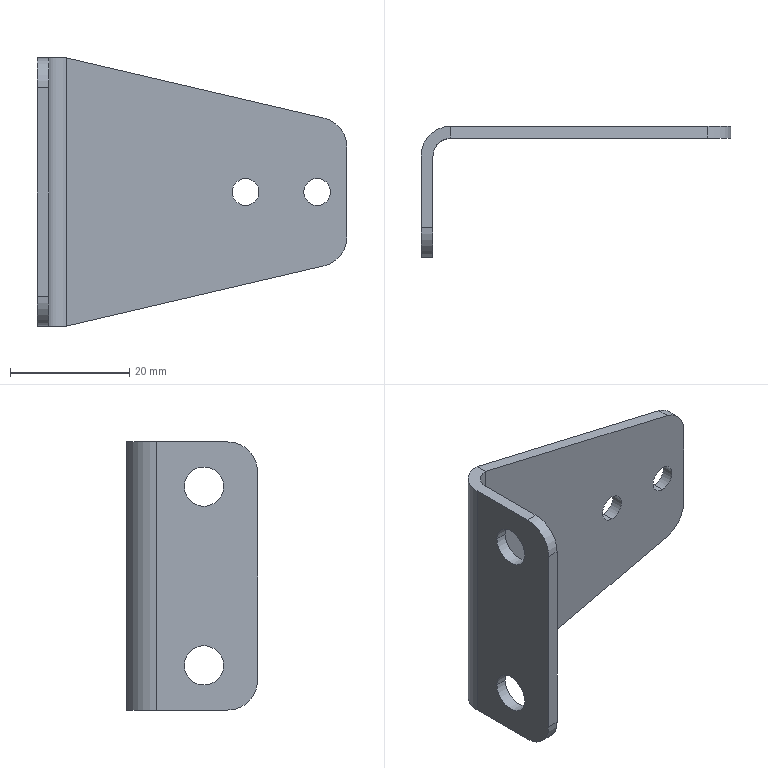Part | SolidWorks | features ICE 3, Extrusion 1, Fillet 1 | 1 solid | 24 faces | box 52 x 22 x 45 mm | volume 5057 mm3 | cylinder 14 | plane 10 | commonest cylinder face diameters 10 x5 4.5 x4 6.6 x4 6 x1
STEP:
#1=CARTESIAN_POINT('',(47.,20.,24.75));
#2=VERTEX_POINT('',#1);
#3=CARTESIAN_POINT('',(47.,20.,20.25));
#4=VERTEX_POINT('',#3);
#5=CARTESIAN_POINT('',(47.,20.,22.5));
#6=DIRECTION('',(0.,-1.,0.));
#7=DIRECTION('',(-1.,0.,0.));
#8=AXIS2_PLACEMENT_3D('',#5,#6,#7);
#9=CIRCLE('',#8,2.25);
#10=EDGE_CURVE('',#2,#4,#9,.T.);
#11=ORIENTED_EDGE('',*,*,#10,.T.);
#12=CARTESIAN_POINT('',(47.,22.,20.25));
#13=VERTEX_POINT('',#12);
#14=CARTESIAN_POINT('',(47.,-0.001,20.25));
#15=DIRECTION('',(0.,1.,0.));
#16=VECTOR('',#15,1000.);
#17=LINE('',#14,#16);
#18=EDGE_CURVE('',#4,#13,#17,.T.);
#19=ORIENTED_EDGE('',*,*,#18,.T.);
#20=CARTESIAN_POINT('',(47.,22.,24.75));
#21=VERTEX_POINT('',#20);
#22=CARTESIAN_POINT('',(47.,22.,22.5));
#23=DIRECTION('',(0.,1.,0.));
#24=DIRECTION('',(0.,0.,1.));
#25=AXIS2_PLACEMENT_3D('',#22,#23,#24);
#26=CIRCLE('',#25,2.25);
#27=EDGE_CURVE('',#13,#21,#26,.T.);
#28=ORIENTED_EDGE('',*,*,#27,.T.);
#29=CARTESIAN_POINT('',(47.,-0.001,24.75));
#30=DIRECTION('',(0.,1.,0.));
#31=VECTOR('',#30,1000.);
#32=LINE('',#29,#31);
#33=EDGE_CURVE('',#2,#21,#32,.T.);
#34=ORIENTED_EDGE('',*,*,#33,.F.);
#35=EDGE_LOOP('',(#11,#19,#28,#34));
#36=FACE_OUTER_BOUND('',#35,.T.);
#37=CARTESIAN_POINT('',(47.,-0.001,22.5));
#38=DIRECTION('',(0.,1.,0.));
#39=DIRECTION('',(0.,0.,1.));
#40=AXIS2_PLACEMENT_3D('',#37,#38,#39);
#41=CYLINDRICAL_SURFACE('',#40,2.25);
#42=ADVANCED_FACE('',(#36),#41,.F.);
#43=CARTESIAN_POINT('',(35.,20.,24.75));
#44=VERTEX_POINT('',#43);
#45=CARTESIAN_POINT('',(35.,20.,20.25));
#46=VERTEX_POINT('',#45);
#47=CARTESIAN_POINT('',(35.,20.,22.5));
#48=DIRECTION('',(0.,-1.,0.));
#49=DIRECTION('',(-1.,0.,0.));
#50=AXIS2_PLACEMENT_3D('',#47,#48,#49);
#51=CIRCLE('',#50,2.25);
#52=EDGE_CURVE('',#44,#46,#51,.T.);
#53=ORIENTED_EDGE('',*,*,#52,.T.);
#54=CARTESIAN_POINT('',(35.,22.,20.25));
#55=VERTEX_POINT('',#54);
#56=CARTESIAN_POINT('',(35.,-0.001,20.25));
#57=DIRECTION('',(0.,1.,0.));
#58=VECTOR('',#57,1000.);
#59=LINE('',#56,#58);
#60=EDGE_CURVE('',#46,#55,#59,.T.);
#61=ORIENTED_EDGE('',*,*,#60,.T.);
#62=CARTESIAN_POINT('',(35.,22.,24.75));
#63=VERTEX_POINT('',#62);
#64=CARTESIAN_POINT('',(35.,22.,22.5));
#65=DIRECTION('',(0.,1.,0.));
#66=DIRECTION('',(0.,0.,1.));
#67=AXIS2_PLACEMENT_3D('',#64,#65,#66);
#68=CIRCLE('',#67,2.25);
#69=EDGE_CURVE('',#55,#63,#68,.T.);
#70=ORIENTED_EDGE('',*,*,#69,.T.);
#71=CARTESIAN_POINT('',(35.,-0.001,24.75));
#72=DIRECTION('',(0.,1.,0.));
#73=VECTOR('',#72,1000.);
#74=LINE('',#71,#73);
#75=EDGE_CURVE('',#44,#63,#74,.T.);
#76=ORIENTED_EDGE('',*,*,#75,.F.);
#77=EDGE_LOOP('',(#53,#61,#70,#76));
#78=FACE_OUTER_BOUND('',#77,.T.);
#79=CARTESIAN_POINT('',(35.,-0.001,22.5));
#80=DIRECTION('',(0.,1.,0.));
#81=DIRECTION('',(0.,0.,1.));
#82=AXIS2_PLACEMENT_3D('',#79,#80,#81);
#83=CYLINDRICAL_SURFACE('',#82,2.25);
#84=ADVANCED_FACE('',(#78),#83,.F.);
#85=CARTESIAN_POINT('',(0.,12.3,7.5));
#86=VERTEX_POINT('',#85);
#87=CARTESIAN_POINT('',(0.,5.7,7.5));
#88=VERTEX_POINT('',#87);
#89=CARTESIAN_POINT('',(0.,9.,7.5));
#90=DIRECTION('',(-1.,0.,0.));
#91=DIRECTION('',(0.,0.,-1.));
#92=AXIS2_PLACEMENT_3D('',#89,#90,#91);
#93=CIRCLE('',#92,3.3);
#94=EDGE_CURVE('',#86,#88,#93,.T.);
#95=ORIENTED_EDGE('',*,*,#94,.T.);
#96=CARTESIAN_POINT('',(2.,5.7,7.5));
#97=VERTEX_POINT('',#96);
#98=CARTESIAN_POINT('',(-0.001,5.7,7.5));
#99=DIRECTION('',(1.,0.,0.));
#100=VECTOR('',#99,1000.);
#101=LINE('',#98,#100);
#102=EDGE_CURVE('',#88,#97,#101,.T.);
#103=ORIENTED_EDGE('',*,*,#102,.T.);
#104=CARTESIAN_POINT('',(2.,12.3,7.5));
#105=VERTEX_POINT('',#104);
#106=CARTESIAN_POINT('',(2.,9.,7.5));
#107=DIRECTION('',(1.,0.,0.));
#108=DIRECTION('',(0.,1.,0.));
#109=AXIS2_PLACEMENT_3D('',#106,#107,#108);
#110=CIRCLE('',#109,3.3);
#111=EDGE_CURVE('',#97,#105,#110,.T.);
#112=ORIENTED_EDGE('',*,*,#111,.T.);
#113=CARTESIAN_POINT('',(-0.001,12.3,7.5));
#114=DIRECTION('',(1.,0.,0.));
#115=VECTOR('',#114,1000.);
#116=LINE('',#113,#115);
#117=EDGE_CURVE('',#86,#105,#116,.T.);
#118=ORIENTED_EDGE('',*,*,#117,.F.);
#119=EDGE_LOOP('',(#95,#103,#112,#118));
#120=FACE_OUTER_BOUND('',#119,.T.);
#121=CARTESIAN_POINT('',(-0.001,9.,7.5));
#122=DIRECTION('',(1.,0.,0.));
#123=DIRECTION('',(0.,1.,0.));
#124=AXIS2_PLACEMENT_3D('',#121,#122,#123);
#125=CYLINDRICAL_SURFACE('',#124,3.3);
#126=ADVANCED_FACE('',(#120),#125,.F.);
#127=CARTESIAN_POINT('',(0.,12.3,37.5));
#128=VERTEX_POINT('',#127);
#129=CARTESIAN_POINT('',(0.,5.7,37.5));
#130=VERTEX_POINT('',#129);
#131=CARTESIAN_POINT('',(0.,9.,37.5));
#132=DIRECTION('',(-1.,0.,0.));
#133=DIRECTION('',(0.,0.,-1.));
#134=AXIS2_PLACEMENT_3D('',#131,#132,#133);
#135=CIRCLE('',#134,3.3);
#136=EDGE_CURVE('',#128,#130,#135,.T.);
#137=ORIENTED_EDGE('',*,*,#136,.T.);
#138=CARTESIAN_POINT('',(2.,5.7,37.5));
#139=VERTEX_POINT('',#138);
#140=CARTESIAN_POINT('',(-0.001,5.7,37.5));
#141=DIRECTION('',(1.,0.,0.));
#142=VECTOR('',#141,1000.);
#143=LINE('',#140,#142);
#144=EDGE_CURVE('',#130,#139,#143,.T.);
#145=ORIENTED_EDGE('',*,*,#144,.T.);
#146=CARTESIAN_POINT('',(2.,12.3,37.5));
#147=VERTEX_POINT('',#146);
#148=CARTESIAN_POINT('',(2.,9.,37.5));
#149=DIRECTION('',(1.,0.,0.));
#150=DIRECTION('',(0.,1.,0.));
#151=AXIS2_PLACEMENT_3D('',#148,#149,#150);
#152=CIRCLE('',#151,3.3);
#153=EDGE_CURVE('',#139,#147,#152,.T.);
#154=ORIENTED_EDGE('',*,*,#153,.T.);
#155=CARTESIAN_POINT('',(-0.001,12.3,37.5));
#156=DIRECTION('',(1.,0.,0.));
#157=VECTOR('',#156,1000.);
#158=LINE('',#155,#157);
#159=EDGE_CURVE('',#128,#147,#158,.T.);
#160=ORIENTED_EDGE('',*,*,#159,.F.);
#161=EDGE_LOOP('',(#137,#145,#154,#160));
#162=FACE_OUTER_BOUND('',#161,.T.);
#163=CARTESIAN_POINT('',(-0.001,9.,37.5));
#164=DIRECTION('',(1.,0.,0.));
#165=DIRECTION('',(0.,1.,0.));
#166=AXIS2_PLACEMENT_3D('',#163,#164,#165);
#167=CYLINDRICAL_SURFACE('',#166,3.3);
#168=ADVANCED_FACE('',(#162),#167,.F.);
#169=CARTESIAN_POINT('',(0.,0.,40.));
#170=VERTEX_POINT('',#169);
#171=CARTESIAN_POINT('',(0.,0.,5.));
#172=VERTEX_POINT('',#171);
#173=CARTESIAN_POINT('',(0.,0.,45.));
#174=DIRECTION('',(0.,0.,-1.));
#175=VECTOR('',#174,1000.);
#176=LINE('',#173,#175);
#177=EDGE_CURVE('',#170,#172,#176,.T.);
#178=ORIENTED_EDGE('',*,*,#177,.T.);
#179=CARTESIAN_POINT('',(2.,0.,5.));
#180=VERTEX_POINT('',#179);
#181=CARTESIAN_POINT('',(2.,0.,5.));
#182=DIRECTION('',(1.,0.,0.));
#183=VECTOR('',#182,1000.);
#184=LINE('',#181,#183);
#185=EDGE_CURVE('',#172,#180,#184,.T.);
#186=ORIENTED_EDGE('',*,*,#185,.T.);
#187=CARTESIAN_POINT('',(2.,0.,40.));
#188=VERTEX_POINT('',#187);
#189=CARTESIAN_POINT('',(2.,0.,45.));
#190=DIRECTION('',(0.,0.,-1.));
#191=VECTOR('',#190,1000.);
#192=LINE('',#189,#191);
#193=EDGE_CURVE('',#188,#180,#192,.T.);
#194=ORIENTED_EDGE('',*,*,#193,.F.);
#195=CARTESIAN_POINT('',(2.,0.,40.));
#196=DIRECTION('',(-1.,0.,0.));
#197=VECTOR('',#196,1000.);
#198=LINE('',#195,#197);
#199=EDGE_CURVE('',#188,#170,#198,.T.);
#200=ORIENTED_EDGE('',*,*,#199,.T.);
#201=EDGE_LOOP('',(#178,#186,#194,#200));
#202=FACE_OUTER_BOUND('',#201,.T.);
#203=CARTESIAN_POINT('',(2.,0.,45.));
#204=DIRECTION('',(0.,1.,0.));
#205=DIRECTION('',(-1.,0.,0.));
#206=AXIS2_PLACEMENT_3D('',#203,#204,#205);
#207=PLANE('',#206);
#208=ADVANCED_FACE('',(#202),#207,.F.);
#209=CARTESIAN_POINT('',(2.,9.,7.5));
#210=DIRECTION('',(1.,0.,0.));
#211=DIRECTION('',(0.,1.,0.));
#212=AXIS2_PLACEMENT_3D('',#209,#210,#211);
#213=CIRCLE('',#212,3.3);
#214=EDGE_CURVE('',#105,#97,#213,.T.);
#215=ORIENTED_EDGE('',*,*,#214,.F.);
#216=ORIENTED_EDGE('',*,*,#111,.F.);
#217=EDGE_LOOP('',(#215,#216));
#218=FACE_BOUND('',#217,.T.);
#219=CARTESIAN_POINT('',(2.,9.,37.5));
#220=DIRECTION('',(1.,0.,0.));
#221=DIRECTION('',(0.,1.,0.));
#222=AXIS2_PLACEMENT_3D('',#219,#220,#221);
#223=CIRCLE('',#222,3.3);
#224=EDGE_CURVE('',#147,#139,#223,.T.);
#225=ORIENTED_EDGE('',*,*,#224,.F.);
#226=ORIENTED_EDGE('',*,*,#153,.F.);
#227=EDGE_LOOP('',(#225,#226));
#228=FACE_BOUND('',#227,.T.);
#229=ORIENTED_EDGE('',*,*,#193,.T.);
#230=CARTESIAN_POINT('',(2.,5.,0.));
#231=VERTEX_POINT('',#230);
#232=CARTESIAN_POINT('',(2.,5.,5.));
#233=DIRECTION('',(1.,0.,0.));
#234=DIRECTION('',(0.,-1.,0.));
#235=AXIS2_PLACEMENT_3D('',#232,#233,#234);
#236=CIRCLE('',#235,5.);
#237=EDGE_CURVE('',#180,#231,#236,.T.);
#238=ORIENTED_EDGE('',*,*,#237,.T.);
#239=CARTESIAN_POINT('',(2.,17.,0.));
#240=VERTEX_POINT('',#239);
#241=CARTESIAN_POINT('',(2.,17.,0.));
#242=DIRECTION('',(0.,1.,0.));
#243=VECTOR('',#242,1000.);
#244=LINE('',#241,#243);
#245=EDGE_CURVE('',#231,#240,#244,.T.);
#246=ORIENTED_EDGE('',*,*,#245,.T.);
#247=CARTESIAN_POINT('',(2.,17.,45.));
#248=VERTEX_POINT('',#247);
#249=CARTESIAN_POINT('',(2.,17.,45.));
#250=DIRECTION('',(0.,0.,-1.));
#251=VECTOR('',#250,1000.);
#252=LINE('',#249,#251);
#253=EDGE_CURVE('',#248,#240,#252,.T.);
#254=ORIENTED_EDGE('',*,*,#253,.F.);
#255=CARTESIAN_POINT('',(2.,5.,45.));
#256=VERTEX_POINT('',#255);
#257=CARTESIAN_POINT('',(2.,17.,45.));
#258=DIRECTION('',(0.,1.,0.));
#259=VECTOR('',#258,1000.);
#260=LINE('',#257,#259);
#261=EDGE_CURVE('',#256,#248,#260,.T.);
#262=ORIENTED_EDGE('',*,*,#261,.F.);
#263=CARTESIAN_POINT('',(2.,5.,40.));
#264=DIRECTION('',(1.,0.,0.));
#265=DIRECTION('',(0.,-1.,0.));
#266=AXIS2_PLACEMENT_3D('',#263,#264,#265);
#267=CIRCLE('',#266,5.);
#268=EDGE_CURVE('',#256,#188,#267,.T.);
#269=ORIENTED_EDGE('',*,*,#268,.T.);
#270=EDGE_LOOP('',(#229,#238,#246,#254,#262,#269));
#271=FACE_OUTER_BOUND('',#270,.T.);
#272=CARTESIAN_POINT('',(2.,17.,45.));
#273=DIRECTION('',(-1.,0.,0.));
#274=DIRECTION('',(0.,-1.,0.));
#275=AXIS2_PLACEMENT_3D('',#272,#273,#274);
#276=PLANE('',#275);
#277=ADVANCED_FACE('',(#218,#228,#271),#276,.F.);
#278=CARTESIAN_POINT('',(5.,20.,0.));
#279=VERTEX_POINT('',#278);
#280=CARTESIAN_POINT('',(5.,17.,0.));
#281=DIRECTION('',(0.,0.,-1.));
#282=DIRECTION('',(1.,0.,0.));
#283=AXIS2_PLACEMENT_3D('',#280,#281,#282);
#284=CIRCLE('',#283,3.);
#285=EDGE_CURVE('',#240,#279,#284,.T.);
#286=ORIENTED_EDGE('',*,*,#285,.T.);
#287=CARTESIAN_POINT('',(5.,20.,45.));
#288=VERTEX_POINT('',#287);
#289=CARTESIAN_POINT('',(5.,20.,45.));
#290=DIRECTION('',(0.,0.,-1.));
#291=VECTOR('',#290,1000.);
#292=LINE('',#289,#291);
#293=EDGE_CURVE('',#288,#279,#292,.T.);
#294=ORIENTED_EDGE('',*,*,#293,.F.);
#295=CARTESIAN_POINT('',(5.,17.,45.));
#296=DIRECTION('',(0.,0.,-1.));
#297=DIRECTION('',(1.,0.,0.));
#298=AXIS2_PLACEMENT_3D('',#295,#296,#297);
#299=CIRCLE('',#298,3.);
#300=EDGE_CURVE('',#248,#288,#299,.T.);
#301=ORIENTED_EDGE('',*,*,#300,.F.);
#302=ORIENTED_EDGE('',*,*,#253,.T.);
#303=EDGE_LOOP('',(#286,#294,#301,#302));
#304=FACE_OUTER_BOUND('',#303,.T.);
#305=CARTESIAN_POINT('',(5.,17.,45.));
#306=DIRECTION('',(0.,0.,-1.));
#307=DIRECTION('',(-1.,0.,0.));
#308=AXIS2_PLACEMENT_3D('',#305,#306,#307);
#309=CYLINDRICAL_SURFACE('',#308,3.);
#310=ADVANCED_FACE('',(#304),#309,.F.);
#311=ORIENTED_EDGE('',*,*,#10,.F.);
#312=CARTESIAN_POINT('',(47.,20.,22.5));
#313=DIRECTION('',(0.,-1.,0.));
#314=DIRECTION('',(-1.,0.,0.));
#315=AXIS2_PLACEMENT_3D('',#312,#313,#314);
#316=CIRCLE('',#315,2.25);
#317=EDGE_CURVE('',#4,#2,#316,.T.);
#318=ORIENTED_EDGE('',*,*,#317,.F.);
#319=EDGE_LOOP('',(#311,#318));
#320=FACE_BOUND('',#319,.T.);
#321=ORIENTED_EDGE('',*,*,#52,.F.);
#322=CARTESIAN_POINT('',(35.,20.,22.5));
#323=DIRECTION('',(0.,-1.,0.));
#324=DIRECTION('',(-1.,0.,0.));
#325=AXIS2_PLACEMENT_3D('',#322,#323,#324);
#326=CIRCLE('',#325,2.25);
#327=EDGE_CURVE('',#46,#44,#326,.T.);
#328=ORIENTED_EDGE('',*,*,#327,.F.);
#329=EDGE_LOOP('',(#321,#328));
#330=FACE_BOUND('',#329,.T.);
#331=CARTESIAN_POINT('',(48.139,20.,10.096));
#332=VERTEX_POINT('',#331);
#333=CARTESIAN_POINT('',(5.,20.,0.));
#334=DIRECTION('',(-0.9737,0.,-0.2279));
#335=VECTOR('',#334,1000.);
#336=LINE('',#333,#335);
#337=EDGE_CURVE('',#332,#279,#336,.T.);
#338=ORIENTED_EDGE('',*,*,#337,.F.);
#339=CARTESIAN_POINT('',(52.,20.,14.965));
#340=VERTEX_POINT('',#339);
#341=CARTESIAN_POINT('',(47.,20.,14.965));
#342=DIRECTION('',(0.,-1.,0.));
#343=DIRECTION('',(-1.,0.,0.));
#344=AXIS2_PLACEMENT_3D('',#341,#342,#343);
#345=CIRCLE('',#344,5.);
#346=EDGE_CURVE('',#332,#340,#345,.T.);
#347=ORIENTED_EDGE('',*,*,#346,.T.);
#348=CARTESIAN_POINT('',(52.,20.,30.035));
#349=VERTEX_POINT('',#348);
#350=CARTESIAN_POINT('',(52.,20.,45.));
#351=DIRECTION('',(0.,0.,-1.));
#352=VECTOR('',#351,1000.);
#353=LINE('',#350,#352);
#354=EDGE_CURVE('',#349,#340,#353,.T.);
#355=ORIENTED_EDGE('',*,*,#354,.F.);
#356=CARTESIAN_POINT('',(48.139,20.,34.904));
#357=VERTEX_POINT('',#356);
#358=CARTESIAN_POINT('',(47.,20.,30.035));
#359=DIRECTION('',(0.,-1.,0.));
#360=DIRECTION('',(-1.,0.,0.));
#361=AXIS2_PLACEMENT_3D('',#358,#359,#360);
#362=CIRCLE('',#361,5.);
#363=EDGE_CURVE('',#349,#357,#362,.T.);
#364=ORIENTED_EDGE('',*,*,#363,.T.);
#365=CARTESIAN_POINT('',(5.,20.,45.));
#366=DIRECTION('',(0.9737,0.,-0.2279));
#367=VECTOR('',#366,1000.);
#368=LINE('',#365,#367);
#369=EDGE_CURVE('',#288,#357,#368,.T.);
#370=ORIENTED_EDGE('',*,*,#369,.F.);
#371=ORIENTED_EDGE('',*,*,#293,.T.);
#372=EDGE_LOOP('',(#338,#347,#355,#364,#370,#371));
#373=FACE_OUTER_BOUND('',#372,.T.);
#374=CARTESIAN_POINT('',(52.,20.,45.));
#375=DIRECTION('',(0.,1.,0.));
#376=DIRECTION('',(-1.,0.,0.));
#377=AXIS2_PLACEMENT_3D('',#374,#375,#376);
#378=PLANE('',#377);
#379=ADVANCED_FACE('',(#320,#330,#373),#378,.F.);
#380=ORIENTED_EDGE('',*,*,#354,.T.);
#381=CARTESIAN_POINT('',(52.,22.,14.965));
#382=VERTEX_POINT('',#381);
#383=CARTESIAN_POINT('',(52.,22.,14.965));
#384=DIRECTION('',(0.,1.,0.));
#385=VECTOR('',#384,1000.);
#386=LINE('',#383,#385);
#387=EDGE_CURVE('',#340,#382,#386,.T.);
#388=ORIENTED_EDGE('',*,*,#387,.T.);
#389=CARTESIAN_POINT('',(52.,22.,30.035));
#390=VERTEX_POINT('',#389);
#391=CARTESIAN_POINT('',(52.,22.,45.));
#392=DIRECTION('',(0.,0.,-1.));
#393=VECTOR('',#392,1000.);
#394=LINE('',#391,#393);
#395=EDGE_CURVE('',#390,#382,#394,.T.);
#396=ORIENTED_EDGE('',*,*,#395,.F.);
#397=CARTESIAN_POINT('',(52.,22.,30.035));
#398=DIRECTION('',(0.,-1.,0.));
#399=VECTOR('',#398,1000.);
#400=LINE('',#397,#399);
#401=EDGE_CURVE('',#390,#349,#400,.T.);
#402=ORIENTED_EDGE('',*,*,#401,.T.);
#403=EDGE_LOOP('',(#380,#388,#396,#402));
#404=FACE_OUTER_BOUND('',#403,.T.);
#405=CARTESIAN_POINT('',(52.,22.,45.));
#406=DIRECTION('',(-1.,0.,0.));
#407=DIRECTION('',(0.,0.,1.));
#408=AXIS2_PLACEMENT_3D('',#405,#406,#407);
#409=PLANE('',#408);
#410=ADVANCED_FACE('',(#404),#409,.F.);
#411=CARTESIAN_POINT('',(47.,22.,22.5));
#412=DIRECTION('',(0.,1.,0.));
#413=DIRECTION('',(0.,0.,1.));
#414=AXIS2_PLACEMENT_3D('',#411,#412,#413);
#415=CIRCLE('',#414,2.25);
#416=EDGE_CURVE('',#21,#13,#415,.T.);
#417=ORIENTED_EDGE('',*,*,#416,.F.);
#418=ORIENTED_EDGE('',*,*,#27,.F.);
#419=EDGE_LOOP('',(#417,#418));
#420=FACE_BOUND('',#419,.T.);
#421=CARTESIAN_POINT('',(35.,22.,22.5));
#422=DIRECTION('',(0.,1.,0.));
#423=DIRECTION('',(0.,0.,1.));
#424=AXIS2_PLACEMENT_3D('',#421,#422,#423);
#425=CIRCLE('',#424,2.25);
#426=EDGE_CURVE('',#63,#55,#425,.T.);
#427=ORIENTED_EDGE('',*,*,#426,.F.);
#428=ORIENTED_EDGE('',*,*,#69,.F.);
#429=EDGE_LOOP('',(#427,#428));
#430=FACE_BOUND('',#429,.T.);
#431=ORIENTED_EDGE('',*,*,#395,.T.);
#432=CARTESIAN_POINT('',(48.139,22.,10.096));
#433=VERTEX_POINT('',#432);
#434=CARTESIAN_POINT('',(47.,22.,14.965));
#435=DIRECTION('',(0.,1.,0.));
#436=DIRECTION('',(1.,0.,0.));
#437=AXIS2_PLACEMENT_3D('',#434,#435,#436);
#438=CIRCLE('',#437,5.);
#439=EDGE_CURVE('',#382,#433,#438,.T.);
#440=ORIENTED_EDGE('',*,*,#439,.T.);
#441=CARTESIAN_POINT('',(5.,22.,0.));
#442=VERTEX_POINT('',#441);
#443=CARTESIAN_POINT('',(5.,22.,0.));
#444=DIRECTION('',(0.9737,0.,0.2279));
#445=VECTOR('',#444,1000.);
#446=LINE('',#443,#445);
#447=EDGE_CURVE('',#442,#433,#446,.T.);
#448=ORIENTED_EDGE('',*,*,#447,.F.);
#449=CARTESIAN_POINT('',(5.,22.,45.));
#450=VERTEX_POINT('',#449);
#451=CARTESIAN_POINT('',(5.,22.,45.));
#452=DIRECTION('',(0.,0.,-1.));
#453=VECTOR('',#452,1000.);
#454=LINE('',#451,#453);
#455=EDGE_CURVE('',#450,#442,#454,.T.);
#456=ORIENTED_EDGE('',*,*,#455,.F.);
#457=CARTESIAN_POINT('',(48.139,22.,34.904));
#458=VERTEX_POINT('',#457);
#459=CARTESIAN_POINT('',(5.,22.,45.));
#460=DIRECTION('',(-0.9737,0.,0.2279));
#461=VECTOR('',#460,1000.);
#462=LINE('',#459,#461);
#463=EDGE_CURVE('',#458,#450,#462,.T.);
#464=ORIENTED_EDGE('',*,*,#463,.F.);
#465=CARTESIAN_POINT('',(47.,22.,30.035));
#466=DIRECTION('',(0.,1.,0.));
#467=DIRECTION('',(1.,0.,0.));
#468=AXIS2_PLACEMENT_3D('',#465,#466,#467);
#469=CIRCLE('',#468,5.);
#470=EDGE_CURVE('',#458,#390,#469,.T.);
#471=ORIENTED_EDGE('',*,*,#470,.T.);
#472=EDGE_LOOP('',(#431,#440,#448,#456,#464,#471));
#473=FACE_OUTER_BOUND('',#472,.T.);
#474=CARTESIAN_POINT('',(5.,22.,45.));
#475=DIRECTION('',(0.,-1.,0.));
#476=DIRECTION('',(1.,0.,0.));
#477=AXIS2_PLACEMENT_3D('',#474,#475,#476);
#478=PLANE('',#477);
#479=ADVANCED_FACE('',(#420,#430,#473),#478,.F.);
#480=CARTESIAN_POINT('',(0.,17.,0.));
#481=VERTEX_POINT('',#480);
#482=CARTESIAN_POINT('',(5.,17.,0.));
#483=DIRECTION('',(0.,0.,1.));
#484=DIRECTION('',(-1.,0.,0.));
#485=AXIS2_PLACEMENT_3D('',#482,#483,#484);
#486=CIRCLE('',#485,5.);
#487=EDGE_CURVE('',#442,#481,#486,.T.);
#488=ORIENTED_EDGE('',*,*,#487,.T.);
#489=CARTESIAN_POINT('',(0.,17.,45.));
#490=VERTEX_POINT('',#489);
#491=CARTESIAN_POINT('',(0.,17.,45.));
#492=DIRECTION('',(0.,0.,-1.));
#493=VECTOR('',#492,1000.);
#494=LINE('',#491,#493);
#495=EDGE_CURVE('',#490,#481,#494,.T.);
#496=ORIENTED_EDGE('',*,*,#495,.F.);
#497=CARTESIAN_POINT('',(5.,17.,45.));
#498=DIRECTION('',(0.,0.,1.));
#499=DIRECTION('',(-1.,0.,0.));
#500=AXIS2_PLACEMENT_3D('',#497,#498,#499);
#501=CIRCLE('',#500,5.);
#502=EDGE_CURVE('',#450,#490,#501,.T.);
#503=ORIENTED_EDGE('',*,*,#502,.F.);
#504=ORIENTED_EDGE('',*,*,#455,.T.);
#505=EDGE_LOOP('',(#488,#496,#503,#504));
#506=FACE_OUTER_BOUND('',#505,.T.);
#507=CARTESIAN_POINT('',(5.,17.,45.));
#508=DIRECTION('',(0.,0.,-1.));
#509=DIRECTION('',(-1.,0.,0.));
#510=AXIS2_PLACEMENT_3D('',#507,#508,#509);
#511=CYLINDRICAL_SURFACE('',#510,5.);
#512=ADVANCED_FACE('',(#506),#511,.T.);
#513=ORIENTED_EDGE('',*,*,#94,.F.);
#514=CARTESIAN_POINT('',(0.,9.,7.5));
#515=DIRECTION('',(-1.,0.,0.));
#516=DIRECTION('',(0.,0.,-1.));
#517=AXIS2_PLACEMENT_3D('',#514,#515,#516);
#518=CIRCLE('',#517,3.3);
#519=EDGE_CURVE('',#88,#86,#518,.T.);
#520=ORIENTED_EDGE('',*,*,#519,.F.);
#521=EDGE_LOOP('',(#513,#520));
#522=FACE_BOUND('',#521,.T.);
#523=ORIENTED_EDGE('',*,*,#136,.F.);
#524=CARTESIAN_POINT('',(0.,9.,37.5));
#525=DIRECTION('',(-1.,0.,0.));
#526=DIRECTION('',(0.,0.,-1.));
#527=AXIS2_PLACEMENT_3D('',#524,#525,#526);
#528=CIRCLE('',#527,3.3);
#529=EDGE_CURVE('',#130,#128,#528,.T.);
#530=ORIENTED_EDGE('',*,*,#529,.F.);
#531=EDGE_LOOP('',(#523,#530));
#532=FACE_BOUND('',#531,.T.);
#533=CARTESIAN_POINT('',(0.,5.,0.));
#534=VERTEX_POINT('',#533);
#535=CARTESIAN_POINT('',(0.,0.,0.));
#536=DIRECTION('',(0.,-1.,0.));
#537=VECTOR('',#536,1000.);
#538=LINE('',#535,#537);
#539=EDGE_CURVE('',#481,#534,#538,.T.);
#540=ORIENTED_EDGE('',*,*,#539,.T.);
#541=CARTESIAN_POINT('',(0.,5.,5.));
#542=DIRECTION('',(-1.,0.,0.));
#543=DIRECTION('',(0.,0.,-1.));
#544=AXIS2_PLACEMENT_3D('',#541,#542,#543);
#545=CIRCLE('',#544,5.);
#546=EDGE_CURVE('',#534,#172,#545,.T.);
#547=ORIENTED_EDGE('',*,*,#546,.T.);
#548=ORIENTED_EDGE('',*,*,#177,.F.);
#549=CARTESIAN_POINT('',(0.,5.,45.));
#550=VERTEX_POINT('',#549);
#551=CARTESIAN_POINT('',(0.,5.,40.));
#552=DIRECTION('',(-1.,0.,0.));
#553=DIRECTION('',(0.,0.,-1.));
#554=AXIS2_PLACEMENT_3D('',#551,#552,#553);
#555=CIRCLE('',#554,5.);
#556=EDGE_CURVE('',#170,#550,#555,.T.);
#557=ORIENTED_EDGE('',*,*,#556,.T.);
#558=CARTESIAN_POINT('',(0.,0.,45.));
#559=DIRECTION('',(0.,-1.,0.));
#560=VECTOR('',#559,1000.);
#561=LINE('',#558,#560);
#562=EDGE_CURVE('',#490,#550,#561,.T.);
#563=ORIENTED_EDGE('',*,*,#562,.F.);
#564=ORIENTED_EDGE('',*,*,#495,.T.);
#565=EDGE_LOOP('',(#540,#547,#548,#557,#563,#564));
#566=FACE_OUTER_BOUND('',#565,.T.);
#567=CARTESIAN_POINT('',(0.,0.,45.));
#568=DIRECTION('',(1.,0.,0.));
#569=DIRECTION('',(0.,0.,-1.));
#570=AXIS2_PLACEMENT_3D('',#567,#568,#569);
#571=PLANE('',#570);
#572=ADVANCED_FACE('',(#522,#532,#566),#571,.F.);
#573=ORIENTED_EDGE('',*,*,#562,.T.);
#574=CARTESIAN_POINT('',(5.,5.,45.));
#575=DIRECTION('',(1.,0.,0.));
#576=VECTOR('',#575,1000.);
#577=LINE('',#574,#576);
#578=EDGE_CURVE('',#550,#256,#577,.T.);
#579=ORIENTED_EDGE('',*,*,#578,.T.);
#580=ORIENTED_EDGE('',*,*,#261,.T.);
#581=ORIENTED_EDGE('',*,*,#300,.T.);
#582=CARTESIAN_POINT('',(5.,-0.001,45.));
#583=DIRECTION('',(0.,1.,0.));
#584=VECTOR('',#583,1000.);
#585=LINE('',#582,#584);
#586=EDGE_CURVE('',#288,#450,#585,.T.);
#587=ORIENTED_EDGE('',*,*,#586,.T.);
#588=ORIENTED_EDGE('',*,*,#502,.T.);
#589=EDGE_LOOP('',(#573,#579,#580,#581,#587,#588));
#590=FACE_OUTER_BOUND('',#589,.T.);
#591=CARTESIAN_POINT('',(5.,17.,45.));
#592=DIRECTION('',(0.,0.,-1.));
#593=DIRECTION('',(-1.,0.,0.));
#594=AXIS2_PLACEMENT_3D('',#591,#592,#593);
#595=PLANE('',#594);
#596=ADVANCED_FACE('',(#590),#595,.F.);
#597=ORIENTED_EDGE('',*,*,#245,.F.);
#598=CARTESIAN_POINT('',(0.,5.,0.));
#599=DIRECTION('',(-1.,0.,0.));
#600=VECTOR('',#599,1000.);
#601=LINE('',#598,#600);
#602=EDGE_CURVE('',#231,#534,#601,.T.);
#603=ORIENTED_EDGE('',*,*,#602,.T.);
#604=ORIENTED_EDGE('',*,*,#539,.F.);
#605=ORIENTED_EDGE('',*,*,#487,.F.);
#606=CARTESIAN_POINT('',(5.,-0.001,0.));
#607=DIRECTION('',(0.,1.,0.));
#608=VECTOR('',#607,1000.);
#609=LINE('',#606,#608);
#610=EDGE_CURVE('',#279,#442,#609,.T.);
#611=ORIENTED_EDGE('',*,*,#610,.F.);
#612=ORIENTED_EDGE('',*,*,#285,.F.);
#613=EDGE_LOOP('',(#597,#603,#604,#605,#611,#612));
#614=FACE_OUTER_BOUND('',#613,.T.);
#615=CARTESIAN_POINT('',(5.,17.,0.));
#616=DIRECTION('',(0.,0.,-1.));
#617=DIRECTION('',(-1.,0.,0.));
#618=AXIS2_PLACEMENT_3D('',#615,#616,#617);
#619=PLANE('',#618);
#620=ADVANCED_FACE('',(#614),#619,.T.);
#621=ORIENTED_EDGE('',*,*,#144,.F.);
#622=ORIENTED_EDGE('',*,*,#529,.T.);
#623=ORIENTED_EDGE('',*,*,#159,.T.);
#624=ORIENTED_EDGE('',*,*,#224,.T.);
#625=EDGE_LOOP('',(#621,#622,#623,#624));
#626=FACE_OUTER_BOUND('',#625,.T.);
#627=CARTESIAN_POINT('',(-0.001,9.,37.5));
#628=DIRECTION('',(1.,0.,0.));
#629=DIRECTION('',(0.,1.,0.));
#630=AXIS2_PLACEMENT_3D('',#627,#628,#629);
#631=CYLINDRICAL_SURFACE('',#630,3.3);
#632=ADVANCED_FACE('',(#626),#631,.F.);
#633=ORIENTED_EDGE('',*,*,#102,.F.);
#634=ORIENTED_EDGE('',*,*,#519,.T.);
#635=ORIENTED_EDGE('',*,*,#117,.T.);
#636=ORIENTED_EDGE('',*,*,#214,.T.);
#637=EDGE_LOOP('',(#633,#634,#635,#636));
#638=FACE_OUTER_BOUND('',#637,.T.);
#639=CARTESIAN_POINT('',(-0.001,9.,7.5));
#640=DIRECTION('',(1.,0.,0.));
#641=DIRECTION('',(0.,1.,0.));
#642=AXIS2_PLACEMENT_3D('',#639,#640,#641);
#643=CYLINDRICAL_SURFACE('',#642,3.3);
#644=ADVANCED_FACE('',(#638),#643,.F.);
#645=ORIENTED_EDGE('',*,*,#60,.F.);
#646=ORIENTED_EDGE('',*,*,#327,.T.);
#647=ORIENTED_EDGE('',*,*,#75,.T.);
#648=ORIENTED_EDGE('',*,*,#426,.T.);
#649=EDGE_LOOP('',(#645,#646,#647,#648));
#650=FACE_OUTER_BOUND('',#649,.T.);
#651=CARTESIAN_POINT('',(35.,-0.001,22.5));
#652=DIRECTION('',(0.,1.,0.));
#653=DIRECTION('',(0.,0.,1.));
#654=AXIS2_PLACEMENT_3D('',#651,#652,#653);
#655=CYLINDRICAL_SURFACE('',#654,2.25);
#656=ADVANCED_FACE('',(#650),#655,.F.);
#657=ORIENTED_EDGE('',*,*,#18,.F.);
#658=ORIENTED_EDGE('',*,*,#317,.T.);
#659=ORIENTED_EDGE('',*,*,#33,.T.);
#660=ORIENTED_EDGE('',*,*,#416,.T.);
#661=EDGE_LOOP('',(#657,#658,#659,#660));
#662=FACE_OUTER_BOUND('',#661,.T.);
#663=CARTESIAN_POINT('',(47.,-0.001,22.5));
#664=DIRECTION('',(0.,1.,0.));
#665=DIRECTION('',(0.,0.,1.));
#666=AXIS2_PLACEMENT_3D('',#663,#664,#665);
#667=CYLINDRICAL_SURFACE('',#666,2.25);
#668=ADVANCED_FACE('',(#662),#667,.F.);
#669=ORIENTED_EDGE('',*,*,#447,.T.);
#670=CARTESIAN_POINT('',(48.139,-0.001,10.096));
#671=DIRECTION('',(0.,-1.,0.));
#672=VECTOR('',#671,1000.);
#673=LINE('',#670,#672);
#674=EDGE_CURVE('',#433,#332,#673,.T.);
#675=ORIENTED_EDGE('',*,*,#674,.T.);
#676=ORIENTED_EDGE('',*,*,#337,.T.);
#677=ORIENTED_EDGE('',*,*,#610,.T.);
#678=EDGE_LOOP('',(#669,#675,#676,#677));
#679=FACE_OUTER_BOUND('',#678,.T.);
#680=CARTESIAN_POINT('',(5.,-0.001,0.));
#681=DIRECTION('',(-0.2279,0.,0.9737));
#682=DIRECTION('',(0.9737,0.,0.2279));
#683=AXIS2_PLACEMENT_3D('',#680,#681,#682);
#684=PLANE('',#683);
#685=ADVANCED_FACE('',(#679),#684,.F.);
#686=ORIENTED_EDGE('',*,*,#369,.T.);
#687=CARTESIAN_POINT('',(48.139,-0.001,34.904));
#688=DIRECTION('',(0.,1.,0.));
#689=VECTOR('',#688,1000.);
#690=LINE('',#687,#689);
#691=EDGE_CURVE('',#357,#458,#690,.T.);
#692=ORIENTED_EDGE('',*,*,#691,.T.);
#693=ORIENTED_EDGE('',*,*,#463,.T.);
#694=ORIENTED_EDGE('',*,*,#586,.F.);
#695=EDGE_LOOP('',(#686,#692,#693,#694));
#696=FACE_OUTER_BOUND('',#695,.T.);
#697=CARTESIAN_POINT('',(5.,-0.001,45.));
#698=DIRECTION('',(-0.2279,0.,-0.9737));
#699=DIRECTION('',(-0.9737,0.,0.2279));
#700=AXIS2_PLACEMENT_3D('',#697,#698,#699);
#701=PLANE('',#700);
#702=ADVANCED_FACE('',(#696),#701,.F.);
#703=ORIENTED_EDGE('',*,*,#546,.F.);
#704=ORIENTED_EDGE('',*,*,#602,.F.);
#705=ORIENTED_EDGE('',*,*,#237,.F.);
#706=ORIENTED_EDGE('',*,*,#185,.F.);
#707=EDGE_LOOP('',(#703,#704,#705,#706));
#708=FACE_OUTER_BOUND('',#707,.T.);
#709=CARTESIAN_POINT('',(2.,5.,5.));
#710=DIRECTION('',(-1.,0.,0.));
#711=DIRECTION('',(0.,-1.,0.));
#712=AXIS2_PLACEMENT_3D('',#709,#710,#711);
#713=CYLINDRICAL_SURFACE('',#712,5.);
#714=ADVANCED_FACE('',(#708),#713,.T.);
#715=ORIENTED_EDGE('',*,*,#556,.F.);
#716=ORIENTED_EDGE('',*,*,#199,.F.);
#717=ORIENTED_EDGE('',*,*,#268,.F.);
#718=ORIENTED_EDGE('',*,*,#578,.F.);
#719=EDGE_LOOP('',(#715,#716,#717,#718));
#720=FACE_OUTER_BOUND('',#719,.T.);
#721=CARTESIAN_POINT('',(5.,5.,40.));
#722=DIRECTION('',(1.,0.,0.));
#723=DIRECTION('',(0.,1.,0.));
#724=AXIS2_PLACEMENT_3D('',#721,#722,#723);
#725=CYLINDRICAL_SURFACE('',#724,5.);
#726=ADVANCED_FACE('',(#720),#725,.T.);
#727=ORIENTED_EDGE('',*,*,#346,.F.);
#728=ORIENTED_EDGE('',*,*,#674,.F.);
#729=ORIENTED_EDGE('',*,*,#439,.F.);
#730=ORIENTED_EDGE('',*,*,#387,.F.);
#731=EDGE_LOOP('',(#727,#728,#729,#730));
#732=FACE_OUTER_BOUND('',#731,.T.);
#733=CARTESIAN_POINT('',(47.,22.,14.965));
#734=DIRECTION('',(0.,1.,0.));
#735=DIRECTION('',(0.,0.,1.));
#736=AXIS2_PLACEMENT_3D('',#733,#734,#735);
#737=CYLINDRICAL_SURFACE('',#736,5.);
#738=ADVANCED_FACE('',(#732),#737,.T.);
#739=ORIENTED_EDGE('',*,*,#363,.F.);
#740=ORIENTED_EDGE('',*,*,#401,.F.);
#741=ORIENTED_EDGE('',*,*,#470,.F.);
#742=ORIENTED_EDGE('',*,*,#691,.F.);
#743=EDGE_LOOP('',(#739,#740,#741,#742));
#744=FACE_OUTER_BOUND('',#743,.T.);
#745=CARTESIAN_POINT('',(47.,-0.001,30.035));
#746=DIRECTION('',(0.,1.,0.));
#747=DIRECTION('',(0.,0.,1.));
#748=AXIS2_PLACEMENT_3D('',#745,#746,#747);
#749=CYLINDRICAL_SURFACE('',#748,5.);
#750=ADVANCED_FACE('',(#744),#749,.T.);
#751=CLOSED_SHELL('',(#42,#84,#126,#168,#208,#277,#310,#379,#410,#479,#512,#572,#596,#620,#632,#644,#656,#668,#685,#702,#714,#726,#738,#750));
#752=MANIFOLD_SOLID_BREP('',#751);
#753=CARTESIAN_POINT('',(0.,0.,0.));
#754=DIRECTION('',(0.,0.,1.));
#755=DIRECTION('',(1.,0.,0.));
#756=AXIS2_PLACEMENT_3D('',#753,#754,#755);
#757=(LENGTH_UNIT()NAMED_UNIT(*)SI_UNIT(.MILLI.,.METRE.));
#758=UNCERTAINTY_MEASURE_WITH_UNIT(LENGTH_MEASURE(0.00001),#757,'','');
#759=(NAMED_UNIT(*)PLANE_ANGLE_UNIT()SI_UNIT($,.RADIAN.));
#760=(NAMED_UNIT(*)SI_UNIT($,.STERADIAN.)SOLID_ANGLE_UNIT());
#761=(GEOMETRIC_REPRESENTATION_CONTEXT(3)GLOBAL_UNCERTAINTY_ASSIGNED_CONTEXT((#758))GLOBAL_UNIT_ASSIGNED_CONTEXT((#757,#759,#760))REPRESENTATION_CONTEXT('',''));
#762=ADVANCED_BREP_SHAPE_REPRESENTATION('',(#752,#756),#761);